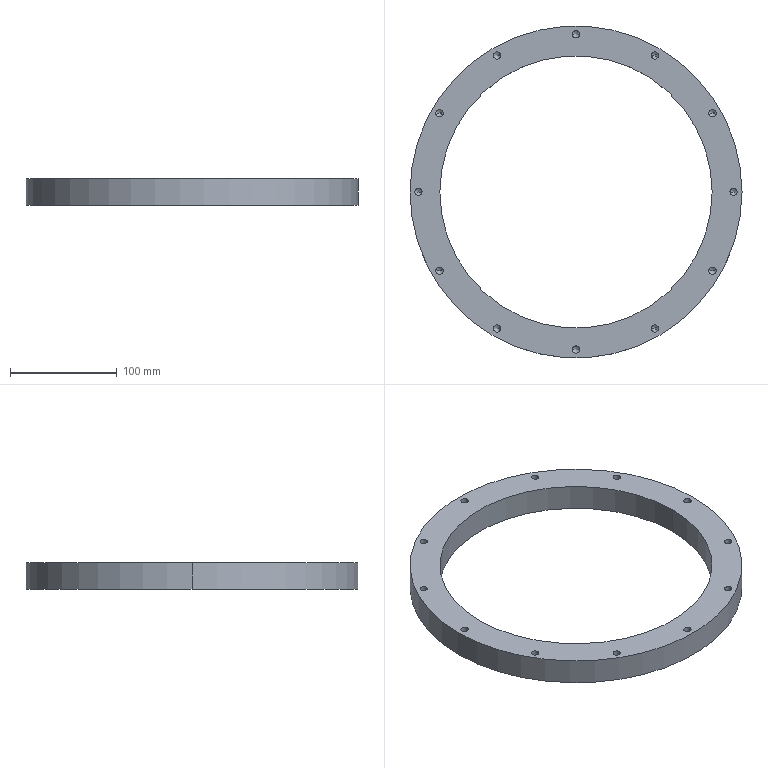Part | STEP file | Bearing connecting disc SGN-2-02 | 1 solid | 54 faces | box 311 x 311 x 25 mm | volume 613337 mm3 | cylinder 28 | cone 24 | plane 2 | commonest cylinder face diameters 6.8 x24 255 x2 311 x2